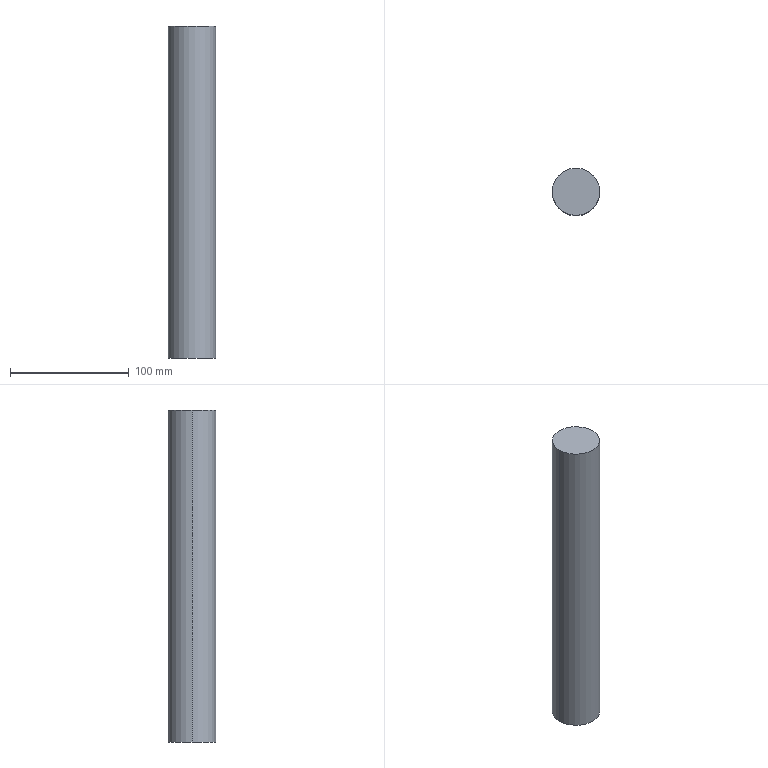Part | SolidWorks | features Extrusion 1 | 1 solid | 4 faces | box 40 x 40 x 280 mm | volume 351858 mm3 | cylinder 2 | plane 2 | commonest cylinder face diameters 40 x2
STEP:
#1=CARTESIAN_POINT('',(20.,0.,250.));
#2=VERTEX_POINT('',#1);
#3=CARTESIAN_POINT('',(-20.,0.,250.));
#4=VERTEX_POINT('',#3);
#5=CARTESIAN_POINT('',(0.,0.,250.));
#6=DIRECTION('',(0.,0.,1.));
#7=DIRECTION('',(1.,0.,0.));
#8=AXIS2_PLACEMENT_3D('',#5,#6,#7);
#9=CIRCLE('',#8,20.);
#10=EDGE_CURVE('',#2,#4,#9,.T.);
#11=ORIENTED_EDGE('',*,*,#10,.F.);
#12=CARTESIAN_POINT('',(20.,0.,-30.));
#13=VERTEX_POINT('',#12);
#14=CARTESIAN_POINT('',(20.,0.,250.));
#15=DIRECTION('',(0.,0.,-1.));
#16=VECTOR('',#15,1000.);
#17=LINE('',#14,#16);
#18=EDGE_CURVE('',#2,#13,#17,.T.);
#19=ORIENTED_EDGE('',*,*,#18,.T.);
#20=CARTESIAN_POINT('',(-20.,0.,-30.));
#21=VERTEX_POINT('',#20);
#22=CARTESIAN_POINT('',(0.,0.,-30.));
#23=DIRECTION('',(0.,0.,1.));
#24=DIRECTION('',(1.,0.,0.));
#25=AXIS2_PLACEMENT_3D('',#22,#23,#24);
#26=CIRCLE('',#25,20.);
#27=EDGE_CURVE('',#13,#21,#26,.T.);
#28=ORIENTED_EDGE('',*,*,#27,.T.);
#29=CARTESIAN_POINT('',(-20.,0.,250.));
#30=DIRECTION('',(0.,0.,-1.));
#31=VECTOR('',#30,1000.);
#32=LINE('',#29,#31);
#33=EDGE_CURVE('',#4,#21,#32,.T.);
#34=ORIENTED_EDGE('',*,*,#33,.F.);
#35=EDGE_LOOP('',(#11,#19,#28,#34));
#36=FACE_OUTER_BOUND('',#35,.T.);
#37=CARTESIAN_POINT('',(0.,0.,250.));
#38=DIRECTION('',(0.,0.,-1.));
#39=DIRECTION('',(-1.,0.,0.));
#40=AXIS2_PLACEMENT_3D('',#37,#38,#39);
#41=CYLINDRICAL_SURFACE('',#40,20.);
#42=ADVANCED_FACE('',(#36),#41,.T.);
#43=ORIENTED_EDGE('',*,*,#18,.F.);
#44=CARTESIAN_POINT('',(0.,0.,250.));
#45=DIRECTION('',(0.,0.,1.));
#46=DIRECTION('',(1.,0.,0.));
#47=AXIS2_PLACEMENT_3D('',#44,#45,#46);
#48=CIRCLE('',#47,20.);
#49=EDGE_CURVE('',#4,#2,#48,.T.);
#50=ORIENTED_EDGE('',*,*,#49,.F.);
#51=ORIENTED_EDGE('',*,*,#33,.T.);
#52=CARTESIAN_POINT('',(0.,0.,-30.));
#53=DIRECTION('',(0.,0.,1.));
#54=DIRECTION('',(1.,0.,0.));
#55=AXIS2_PLACEMENT_3D('',#52,#53,#54);
#56=CIRCLE('',#55,20.);
#57=EDGE_CURVE('',#21,#13,#56,.T.);
#58=ORIENTED_EDGE('',*,*,#57,.T.);
#59=EDGE_LOOP('',(#43,#50,#51,#58));
#60=FACE_OUTER_BOUND('',#59,.T.);
#61=CARTESIAN_POINT('',(0.,0.,250.));
#62=DIRECTION('',(0.,0.,-1.));
#63=DIRECTION('',(-1.,0.,0.));
#64=AXIS2_PLACEMENT_3D('',#61,#62,#63);
#65=CYLINDRICAL_SURFACE('',#64,20.);
#66=ADVANCED_FACE('',(#60),#65,.T.);
#67=ORIENTED_EDGE('',*,*,#49,.T.);
#68=ORIENTED_EDGE('',*,*,#10,.T.);
#69=EDGE_LOOP('',(#67,#68));
#70=FACE_OUTER_BOUND('',#69,.T.);
#71=CARTESIAN_POINT('',(0.,0.,250.));
#72=DIRECTION('',(0.,0.,1.));
#73=DIRECTION('',(1.,0.,0.));
#74=AXIS2_PLACEMENT_3D('',#71,#72,#73);
#75=PLANE('',#74);
#76=ADVANCED_FACE('',(#70),#75,.T.);
#77=ORIENTED_EDGE('',*,*,#57,.F.);
#78=ORIENTED_EDGE('',*,*,#27,.F.);
#79=EDGE_LOOP('',(#77,#78));
#80=FACE_OUTER_BOUND('',#79,.T.);
#81=CARTESIAN_POINT('',(0.,0.,-30.));
#82=DIRECTION('',(0.,0.,1.));
#83=DIRECTION('',(1.,0.,0.));
#84=AXIS2_PLACEMENT_3D('',#81,#82,#83);
#85=PLANE('',#84);
#86=ADVANCED_FACE('',(#80),#85,.F.);
#87=CLOSED_SHELL('',(#42,#66,#76,#86));
#88=MANIFOLD_SOLID_BREP('',#87);
#89=CARTESIAN_POINT('',(0.,0.,0.));
#90=DIRECTION('',(0.,0.,1.));
#91=DIRECTION('',(1.,0.,0.));
#92=AXIS2_PLACEMENT_3D('',#89,#90,#91);
#93=(LENGTH_UNIT()NAMED_UNIT(*)SI_UNIT(.MILLI.,.METRE.));
#94=UNCERTAINTY_MEASURE_WITH_UNIT(LENGTH_MEASURE(0.00001),#93,'','');
#95=(NAMED_UNIT(*)PLANE_ANGLE_UNIT()SI_UNIT($,.RADIAN.));
#96=(NAMED_UNIT(*)SI_UNIT($,.STERADIAN.)SOLID_ANGLE_UNIT());
#97=(GEOMETRIC_REPRESENTATION_CONTEXT(3)GLOBAL_UNCERTAINTY_ASSIGNED_CONTEXT((#94))GLOBAL_UNIT_ASSIGNED_CONTEXT((#93,#95,#96))REPRESENTATION_CONTEXT('',''));
#98=ADVANCED_BREP_SHAPE_REPRESENTATION('',(#88,#92),#97);